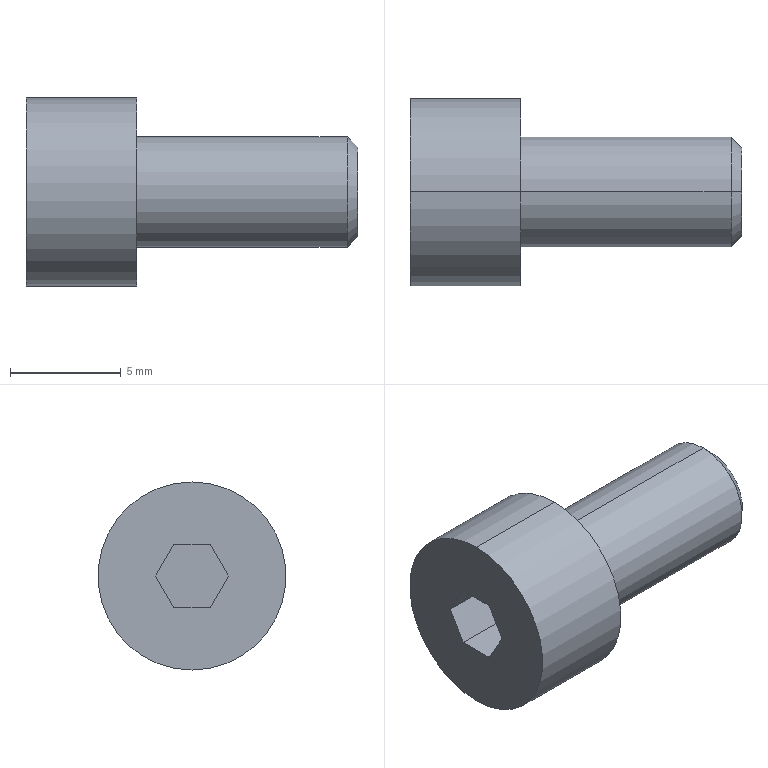Part | STEP file | _DBA01-D50-d20-e22-005 | 1 solid | 16 faces | box 15 x 8.5 x 8.5 mm | volume 460.635 mm3 | plane 10 | cylinder 4 | cone 2 | commonest cylinder face diameters 5 x2 8.5 x2
STEP:
#1=CARTESIAN_POINT('',(5.,0.,-2.5));
#2=VERTEX_POINT('',#1);
#3=CARTESIAN_POINT('',(5.,0.,2.5));
#4=VERTEX_POINT('',#3);
#5=CARTESIAN_POINT('',(5.,0.,0.));
#6=DIRECTION('',(-1.,0.,0.));
#7=DIRECTION('',(0.,0.,1.));
#8=AXIS2_PLACEMENT_3D('',#5,#6,#7);
#9=CIRCLE('',#8,2.5);
#10=EDGE_CURVE('',#2,#4,#9,.T.);
#11=ORIENTED_EDGE('',*,*,#10,.F.);
#12=CARTESIAN_POINT('',(14.509,0.,-2.5));
#13=VERTEX_POINT('',#12);
#14=CARTESIAN_POINT('',(0.,0.,-2.5));
#15=DIRECTION('',(1.,0.,0.));
#16=VECTOR('',#15,1000.);
#17=LINE('',#14,#16);
#18=EDGE_CURVE('',#2,#13,#17,.T.);
#19=ORIENTED_EDGE('',*,*,#18,.T.);
#20=CARTESIAN_POINT('',(14.509,0.,2.5));
#21=VERTEX_POINT('',#20);
#22=CARTESIAN_POINT('',(14.509,0.,0.));
#23=DIRECTION('',(-1.,0.,0.));
#24=DIRECTION('',(0.,0.,1.));
#25=AXIS2_PLACEMENT_3D('',#22,#23,#24);
#26=CIRCLE('',#25,2.5);
#27=EDGE_CURVE('',#13,#21,#26,.T.);
#28=ORIENTED_EDGE('',*,*,#27,.T.);
#29=CARTESIAN_POINT('',(0.,0.,2.5));
#30=DIRECTION('',(1.,0.,0.));
#31=VECTOR('',#30,1000.);
#32=LINE('',#29,#31);
#33=EDGE_CURVE('',#4,#21,#32,.T.);
#34=ORIENTED_EDGE('',*,*,#33,.F.);
#35=EDGE_LOOP('',(#11,#19,#28,#34));
#36=FACE_OUTER_BOUND('',#35,.T.);
#37=CARTESIAN_POINT('',(0.,0.,0.));
#38=DIRECTION('',(1.,0.,0.));
#39=DIRECTION('',(0.,0.,1.));
#40=AXIS2_PLACEMENT_3D('',#37,#38,#39);
#41=CYLINDRICAL_SURFACE('',#40,2.5);
#42=ADVANCED_FACE('',(#36),#41,.T.);
#43=CARTESIAN_POINT('',(0.,0.,-4.25));
#44=VERTEX_POINT('',#43);
#45=CARTESIAN_POINT('',(0.,0.,4.25));
#46=VERTEX_POINT('',#45);
#47=CARTESIAN_POINT('',(0.,0.,0.));
#48=DIRECTION('',(-1.,0.,0.));
#49=DIRECTION('',(0.,0.,1.));
#50=AXIS2_PLACEMENT_3D('',#47,#48,#49);
#51=CIRCLE('',#50,4.25);
#52=EDGE_CURVE('',#44,#46,#51,.T.);
#53=ORIENTED_EDGE('',*,*,#52,.F.);
#54=CARTESIAN_POINT('',(5.,0.,-4.25));
#55=VERTEX_POINT('',#54);
#56=CARTESIAN_POINT('',(0.,0.,-4.25));
#57=DIRECTION('',(1.,0.,0.));
#58=VECTOR('',#57,1000.);
#59=LINE('',#56,#58);
#60=EDGE_CURVE('',#44,#55,#59,.T.);
#61=ORIENTED_EDGE('',*,*,#60,.T.);
#62=CARTESIAN_POINT('',(5.,0.,4.25));
#63=VERTEX_POINT('',#62);
#64=CARTESIAN_POINT('',(5.,0.,0.));
#65=DIRECTION('',(-1.,0.,0.));
#66=DIRECTION('',(0.,0.,1.));
#67=AXIS2_PLACEMENT_3D('',#64,#65,#66);
#68=CIRCLE('',#67,4.25);
#69=EDGE_CURVE('',#55,#63,#68,.T.);
#70=ORIENTED_EDGE('',*,*,#69,.T.);
#71=CARTESIAN_POINT('',(0.,0.,4.25));
#72=DIRECTION('',(1.,0.,0.));
#73=VECTOR('',#72,1000.);
#74=LINE('',#71,#73);
#75=EDGE_CURVE('',#46,#63,#74,.T.);
#76=ORIENTED_EDGE('',*,*,#75,.F.);
#77=EDGE_LOOP('',(#53,#61,#70,#76));
#78=FACE_OUTER_BOUND('',#77,.T.);
#79=CARTESIAN_POINT('',(0.,0.,0.));
#80=DIRECTION('',(1.,0.,0.));
#81=DIRECTION('',(0.,0.,1.));
#82=AXIS2_PLACEMENT_3D('',#79,#80,#81);
#83=CYLINDRICAL_SURFACE('',#82,4.25);
#84=ADVANCED_FACE('',(#78),#83,.T.);
#85=CARTESIAN_POINT('',(15.,0.,2.01));
#86=VERTEX_POINT('',#85);
#87=CARTESIAN_POINT('',(15.,0.,-2.01));
#88=VERTEX_POINT('',#87);
#89=CARTESIAN_POINT('',(15.,0.,0.));
#90=DIRECTION('',(-1.,0.,0.));
#91=DIRECTION('',(0.,0.,1.));
#92=AXIS2_PLACEMENT_3D('',#89,#90,#91);
#93=CIRCLE('',#92,2.01);
#94=EDGE_CURVE('',#86,#88,#93,.T.);
#95=ORIENTED_EDGE('',*,*,#94,.T.);
#96=CARTESIAN_POINT('',(15.,0.,-2.01));
#97=DIRECTION('',(-0.7071,0.,-0.7071));
#98=VECTOR('',#97,1000.);
#99=LINE('',#96,#98);
#100=EDGE_CURVE('',#88,#13,#99,.T.);
#101=ORIENTED_EDGE('',*,*,#100,.T.);
#102=CARTESIAN_POINT('',(14.509,0.,0.));
#103=DIRECTION('',(-1.,0.,0.));
#104=DIRECTION('',(0.,0.,1.));
#105=AXIS2_PLACEMENT_3D('',#102,#103,#104);
#106=CIRCLE('',#105,2.5);
#107=EDGE_CURVE('',#21,#13,#106,.T.);
#108=ORIENTED_EDGE('',*,*,#107,.F.);
#109=CARTESIAN_POINT('',(15.,0.,2.01));
#110=DIRECTION('',(-0.7071,0.,0.7071));
#111=VECTOR('',#110,1000.);
#112=LINE('',#109,#111);
#113=EDGE_CURVE('',#86,#21,#112,.T.);
#114=ORIENTED_EDGE('',*,*,#113,.F.);
#115=EDGE_LOOP('',(#95,#101,#108,#114));
#116=FACE_OUTER_BOUND('',#115,.T.);
#117=CARTESIAN_POINT('',(15.,0.,0.));
#118=DIRECTION('',(-1.,0.,0.));
#119=DIRECTION('',(0.,0.,1.));
#120=AXIS2_PLACEMENT_3D('',#117,#118,#119);
#121=CONICAL_SURFACE('',#120,2.01,0.7854);
#122=ADVANCED_FACE('',(#116),#121,.T.);
#123=ORIENTED_EDGE('',*,*,#100,.F.);
#124=CARTESIAN_POINT('',(15.,0.,0.));
#125=DIRECTION('',(-1.,0.,0.));
#126=DIRECTION('',(0.,0.,1.));
#127=AXIS2_PLACEMENT_3D('',#124,#125,#126);
#128=CIRCLE('',#127,2.01);
#129=EDGE_CURVE('',#88,#86,#128,.T.);
#130=ORIENTED_EDGE('',*,*,#129,.T.);
#131=ORIENTED_EDGE('',*,*,#113,.T.);
#132=ORIENTED_EDGE('',*,*,#27,.F.);
#133=EDGE_LOOP('',(#123,#130,#131,#132));
#134=FACE_OUTER_BOUND('',#133,.T.);
#135=CARTESIAN_POINT('',(15.,0.,0.));
#136=DIRECTION('',(-1.,0.,0.));
#137=DIRECTION('',(0.,0.,1.));
#138=AXIS2_PLACEMENT_3D('',#135,#136,#137);
#139=CONICAL_SURFACE('',#138,2.01,0.7854);
#140=ADVANCED_FACE('',(#134),#139,.T.);
#141=ORIENTED_EDGE('',*,*,#94,.F.);
#142=ORIENTED_EDGE('',*,*,#129,.F.);
#143=EDGE_LOOP('',(#141,#142));
#144=FACE_OUTER_BOUND('',#143,.T.);
#145=CARTESIAN_POINT('',(15.,0.,0.));
#146=DIRECTION('',(-1.,0.,0.));
#147=DIRECTION('',(0.,0.,1.));
#148=AXIS2_PLACEMENT_3D('',#145,#146,#147);
#149=PLANE('',#148);
#150=ADVANCED_FACE('',(#144),#149,.F.);
#151=CARTESIAN_POINT('',(0.,0.,0.));
#152=DIRECTION('',(-1.,0.,0.));
#153=DIRECTION('',(0.,0.,1.));
#154=AXIS2_PLACEMENT_3D('',#151,#152,#153);
#155=CIRCLE('',#154,4.25);
#156=EDGE_CURVE('',#46,#44,#155,.T.);
#157=ORIENTED_EDGE('',*,*,#156,.T.);
#158=ORIENTED_EDGE('',*,*,#52,.T.);
#159=EDGE_LOOP('',(#157,#158));
#160=FACE_OUTER_BOUND('',#159,.T.);
#161=CARTESIAN_POINT('',(0.,-0.8248,1.429));
#162=VERTEX_POINT('',#161);
#163=CARTESIAN_POINT('',(0.,-1.65,0.));
#164=VERTEX_POINT('',#163);
#165=CARTESIAN_POINT('',(0.,-0.8248,1.429));
#166=DIRECTION('',(0.,-0.5,-0.866));
#167=VECTOR('',#166,1000.);
#168=LINE('',#165,#167);
#169=EDGE_CURVE('',#162,#164,#168,.T.);
#170=ORIENTED_EDGE('',*,*,#169,.T.);
#171=CARTESIAN_POINT('',(0.,-0.8248,-1.429));
#172=VERTEX_POINT('',#171);
#173=CARTESIAN_POINT('',(0.,-1.65,0.));
#174=DIRECTION('',(0.,0.5,-0.866));
#175=VECTOR('',#174,1000.);
#176=LINE('',#173,#175);
#177=EDGE_CURVE('',#164,#172,#176,.T.);
#178=ORIENTED_EDGE('',*,*,#177,.T.);
#179=CARTESIAN_POINT('',(0.,0.8248,-1.429));
#180=VERTEX_POINT('',#179);
#181=CARTESIAN_POINT('',(0.,-0.8248,-1.429));
#182=DIRECTION('',(0.,1.,0.));
#183=VECTOR('',#182,1000.);
#184=LINE('',#181,#183);
#185=EDGE_CURVE('',#172,#180,#184,.T.);
#186=ORIENTED_EDGE('',*,*,#185,.T.);
#187=CARTESIAN_POINT('',(0.,1.65,0.));
#188=VERTEX_POINT('',#187);
#189=CARTESIAN_POINT('',(0.,0.8248,-1.429));
#190=DIRECTION('',(0.,0.5,0.866));
#191=VECTOR('',#190,1000.);
#192=LINE('',#189,#191);
#193=EDGE_CURVE('',#180,#188,#192,.T.);
#194=ORIENTED_EDGE('',*,*,#193,.T.);
#195=CARTESIAN_POINT('',(0.,0.8248,1.429));
#196=VERTEX_POINT('',#195);
#197=CARTESIAN_POINT('',(0.,1.65,0.));
#198=DIRECTION('',(0.,-0.5,0.866));
#199=VECTOR('',#198,1000.);
#200=LINE('',#197,#199);
#201=EDGE_CURVE('',#188,#196,#200,.T.);
#202=ORIENTED_EDGE('',*,*,#201,.T.);
#203=CARTESIAN_POINT('',(0.,0.8248,1.429));
#204=DIRECTION('',(0.,-1.,0.));
#205=VECTOR('',#204,1000.);
#206=LINE('',#203,#205);
#207=EDGE_CURVE('',#196,#162,#206,.T.);
#208=ORIENTED_EDGE('',*,*,#207,.T.);
#209=EDGE_LOOP('',(#170,#178,#186,#194,#202,#208));
#210=FACE_BOUND('',#209,.T.);
#211=CARTESIAN_POINT('',(0.,-4.25,0.));
#212=DIRECTION('',(1.,0.,0.));
#213=DIRECTION('',(0.,1.,0.));
#214=AXIS2_PLACEMENT_3D('',#211,#212,#213);
#215=PLANE('',#214);
#216=ADVANCED_FACE('',(#160,#210),#215,.F.);
#217=ORIENTED_EDGE('',*,*,#60,.F.);
#218=ORIENTED_EDGE('',*,*,#156,.F.);
#219=ORIENTED_EDGE('',*,*,#75,.T.);
#220=CARTESIAN_POINT('',(5.,0.,0.));
#221=DIRECTION('',(-1.,0.,0.));
#222=DIRECTION('',(0.,0.,1.));
#223=AXIS2_PLACEMENT_3D('',#220,#221,#222);
#224=CIRCLE('',#223,4.25);
#225=EDGE_CURVE('',#63,#55,#224,.T.);
#226=ORIENTED_EDGE('',*,*,#225,.T.);
#227=EDGE_LOOP('',(#217,#218,#219,#226));
#228=FACE_OUTER_BOUND('',#227,.T.);
#229=CARTESIAN_POINT('',(0.,0.,0.));
#230=DIRECTION('',(1.,0.,0.));
#231=DIRECTION('',(0.,0.,1.));
#232=AXIS2_PLACEMENT_3D('',#229,#230,#231);
#233=CYLINDRICAL_SURFACE('',#232,4.25);
#234=ADVANCED_FACE('',(#228),#233,.T.);
#235=ORIENTED_EDGE('',*,*,#225,.F.);
#236=ORIENTED_EDGE('',*,*,#69,.F.);
#237=EDGE_LOOP('',(#235,#236));
#238=FACE_OUTER_BOUND('',#237,.T.);
#239=CARTESIAN_POINT('',(5.,0.,0.));
#240=DIRECTION('',(-1.,0.,0.));
#241=DIRECTION('',(0.,0.,1.));
#242=AXIS2_PLACEMENT_3D('',#239,#240,#241);
#243=CIRCLE('',#242,2.5);
#244=EDGE_CURVE('',#4,#2,#243,.T.);
#245=ORIENTED_EDGE('',*,*,#244,.T.);
#246=ORIENTED_EDGE('',*,*,#10,.T.);
#247=EDGE_LOOP('',(#245,#246));
#248=FACE_BOUND('',#247,.T.);
#249=CARTESIAN_POINT('',(5.,-2.5,0.));
#250=DIRECTION('',(-1.,0.,0.));
#251=DIRECTION('',(0.,0.,1.));
#252=AXIS2_PLACEMENT_3D('',#249,#250,#251);
#253=PLANE('',#252);
#254=ADVANCED_FACE('',(#238,#248),#253,.F.);
#255=ORIENTED_EDGE('',*,*,#18,.F.);
#256=ORIENTED_EDGE('',*,*,#244,.F.);
#257=ORIENTED_EDGE('',*,*,#33,.T.);
#258=ORIENTED_EDGE('',*,*,#107,.T.);
#259=EDGE_LOOP('',(#255,#256,#257,#258));
#260=FACE_OUTER_BOUND('',#259,.T.);
#261=CARTESIAN_POINT('',(0.,0.,0.));
#262=DIRECTION('',(1.,0.,0.));
#263=DIRECTION('',(0.,0.,1.));
#264=AXIS2_PLACEMENT_3D('',#261,#262,#263);
#265=CYLINDRICAL_SURFACE('',#264,2.5);
#266=ADVANCED_FACE('',(#260),#265,.T.);
#267=ORIENTED_EDGE('',*,*,#207,.F.);
#268=CARTESIAN_POINT('',(2.5,0.8248,1.429));
#269=VERTEX_POINT('',#268);
#270=CARTESIAN_POINT('',(2.5,0.8248,1.429));
#271=DIRECTION('',(-1.,0.,0.));
#272=VECTOR('',#271,1000.);
#273=LINE('',#270,#272);
#274=EDGE_CURVE('',#269,#196,#273,.T.);
#275=ORIENTED_EDGE('',*,*,#274,.F.);
#276=CARTESIAN_POINT('',(2.5,-0.8248,1.429));
#277=VERTEX_POINT('',#276);
#278=CARTESIAN_POINT('',(2.5,0.8248,1.429));
#279=DIRECTION('',(0.,-1.,0.));
#280=VECTOR('',#279,1000.);
#281=LINE('',#278,#280);
#282=EDGE_CURVE('',#269,#277,#281,.T.);
#283=ORIENTED_EDGE('',*,*,#282,.T.);
#284=CARTESIAN_POINT('',(2.5,-0.8248,1.429));
#285=DIRECTION('',(-1.,0.,0.));
#286=VECTOR('',#285,1000.);
#287=LINE('',#284,#286);
#288=EDGE_CURVE('',#277,#162,#287,.T.);
#289=ORIENTED_EDGE('',*,*,#288,.T.);
#290=EDGE_LOOP('',(#267,#275,#283,#289));
#291=FACE_OUTER_BOUND('',#290,.T.);
#292=CARTESIAN_POINT('',(2.5,0.8248,1.429));
#293=DIRECTION('',(0.,0.,-1.));
#294=DIRECTION('',(0.,-1.,0.));
#295=AXIS2_PLACEMENT_3D('',#292,#293,#294);
#296=PLANE('',#295);
#297=ADVANCED_FACE('',(#291),#296,.T.);
#298=ORIENTED_EDGE('',*,*,#169,.F.);
#299=ORIENTED_EDGE('',*,*,#288,.F.);
#300=CARTESIAN_POINT('',(2.5,-1.65,0.));
#301=VERTEX_POINT('',#300);
#302=CARTESIAN_POINT('',(2.5,-0.8248,1.429));
#303=DIRECTION('',(0.,-0.5,-0.866));
#304=VECTOR('',#303,1000.);
#305=LINE('',#302,#304);
#306=EDGE_CURVE('',#277,#301,#305,.T.);
#307=ORIENTED_EDGE('',*,*,#306,.T.);
#308=CARTESIAN_POINT('',(2.5,-1.65,0.));
#309=DIRECTION('',(-1.,0.,0.));
#310=VECTOR('',#309,1000.);
#311=LINE('',#308,#310);
#312=EDGE_CURVE('',#301,#164,#311,.T.);
#313=ORIENTED_EDGE('',*,*,#312,.T.);
#314=EDGE_LOOP('',(#298,#299,#307,#313));
#315=FACE_OUTER_BOUND('',#314,.T.);
#316=CARTESIAN_POINT('',(2.5,-0.8248,1.429));
#317=DIRECTION('',(0.,0.866,-0.5));
#318=DIRECTION('',(-1.,0.,0.));
#319=AXIS2_PLACEMENT_3D('',#316,#317,#318);
#320=PLANE('',#319);
#321=ADVANCED_FACE('',(#315),#320,.T.);
#322=ORIENTED_EDGE('',*,*,#177,.F.);
#323=ORIENTED_EDGE('',*,*,#312,.F.);
#324=CARTESIAN_POINT('',(2.5,-0.8248,-1.429));
#325=VERTEX_POINT('',#324);
#326=CARTESIAN_POINT('',(2.5,-1.65,0.));
#327=DIRECTION('',(0.,0.5,-0.866));
#328=VECTOR('',#327,1000.);
#329=LINE('',#326,#328);
#330=EDGE_CURVE('',#301,#325,#329,.T.);
#331=ORIENTED_EDGE('',*,*,#330,.T.);
#332=CARTESIAN_POINT('',(2.5,-0.8248,-1.429));
#333=DIRECTION('',(-1.,0.,0.));
#334=VECTOR('',#333,1000.);
#335=LINE('',#332,#334);
#336=EDGE_CURVE('',#325,#172,#335,.T.);
#337=ORIENTED_EDGE('',*,*,#336,.T.);
#338=EDGE_LOOP('',(#322,#323,#331,#337));
#339=FACE_OUTER_BOUND('',#338,.T.);
#340=CARTESIAN_POINT('',(2.5,-1.65,0.));
#341=DIRECTION('',(0.,0.866,0.5));
#342=DIRECTION('',(1.,0.,0.));
#343=AXIS2_PLACEMENT_3D('',#340,#341,#342);
#344=PLANE('',#343);
#345=ADVANCED_FACE('',(#339),#344,.T.);
#346=ORIENTED_EDGE('',*,*,#185,.F.);
#347=ORIENTED_EDGE('',*,*,#336,.F.);
#348=CARTESIAN_POINT('',(2.5,0.8248,-1.429));
#349=VERTEX_POINT('',#348);
#350=CARTESIAN_POINT('',(2.5,-0.8248,-1.429));
#351=DIRECTION('',(0.,1.,0.));
#352=VECTOR('',#351,1000.);
#353=LINE('',#350,#352);
#354=EDGE_CURVE('',#325,#349,#353,.T.);
#355=ORIENTED_EDGE('',*,*,#354,.T.);
#356=CARTESIAN_POINT('',(2.5,0.8248,-1.429));
#357=DIRECTION('',(-1.,0.,0.));
#358=VECTOR('',#357,1000.);
#359=LINE('',#356,#358);
#360=EDGE_CURVE('',#349,#180,#359,.T.);
#361=ORIENTED_EDGE('',*,*,#360,.T.);
#362=EDGE_LOOP('',(#346,#347,#355,#361));
#363=FACE_OUTER_BOUND('',#362,.T.);
#364=CARTESIAN_POINT('',(2.5,-0.8248,-1.429));
#365=DIRECTION('',(0.,0.,1.));
#366=DIRECTION('',(1.,0.,0.));
#367=AXIS2_PLACEMENT_3D('',#364,#365,#366);
#368=PLANE('',#367);
#369=ADVANCED_FACE('',(#363),#368,.T.);
#370=ORIENTED_EDGE('',*,*,#193,.F.);
#371=ORIENTED_EDGE('',*,*,#360,.F.);
#372=CARTESIAN_POINT('',(2.5,1.65,0.));
#373=VERTEX_POINT('',#372);
#374=CARTESIAN_POINT('',(2.5,0.8248,-1.429));
#375=DIRECTION('',(0.,0.5,0.866));
#376=VECTOR('',#375,1000.);
#377=LINE('',#374,#376);
#378=EDGE_CURVE('',#349,#373,#377,.T.);
#379=ORIENTED_EDGE('',*,*,#378,.T.);
#380=CARTESIAN_POINT('',(2.5,1.65,0.));
#381=DIRECTION('',(-1.,0.,0.));
#382=VECTOR('',#381,1000.);
#383=LINE('',#380,#382);
#384=EDGE_CURVE('',#373,#188,#383,.T.);
#385=ORIENTED_EDGE('',*,*,#384,.T.);
#386=EDGE_LOOP('',(#370,#371,#379,#385));
#387=FACE_OUTER_BOUND('',#386,.T.);
#388=CARTESIAN_POINT('',(2.5,0.8248,-1.429));
#389=DIRECTION('',(0.,-0.866,0.5));
#390=DIRECTION('',(-1.,0.,0.));
#391=AXIS2_PLACEMENT_3D('',#388,#389,#390);
#392=PLANE('',#391);
#393=ADVANCED_FACE('',(#387),#392,.T.);
#394=ORIENTED_EDGE('',*,*,#201,.F.);
#395=ORIENTED_EDGE('',*,*,#384,.F.);
#396=CARTESIAN_POINT('',(2.5,1.65,0.));
#397=DIRECTION('',(0.,-0.5,0.866));
#398=VECTOR('',#397,1000.);
#399=LINE('',#396,#398);
#400=EDGE_CURVE('',#373,#269,#399,.T.);
#401=ORIENTED_EDGE('',*,*,#400,.T.);
#402=ORIENTED_EDGE('',*,*,#274,.T.);
#403=EDGE_LOOP('',(#394,#395,#401,#402));
#404=FACE_OUTER_BOUND('',#403,.T.);
#405=CARTESIAN_POINT('',(2.5,1.65,0.));
#406=DIRECTION('',(0.,-0.866,-0.5));
#407=DIRECTION('',(0.,0.5,-0.866));
#408=AXIS2_PLACEMENT_3D('',#405,#406,#407);
#409=PLANE('',#408);
#410=ADVANCED_FACE('',(#404),#409,.T.);
#411=ORIENTED_EDGE('',*,*,#282,.F.);
#412=ORIENTED_EDGE('',*,*,#400,.F.);
#413=ORIENTED_EDGE('',*,*,#378,.F.);
#414=ORIENTED_EDGE('',*,*,#354,.F.);
#415=ORIENTED_EDGE('',*,*,#330,.F.);
#416=ORIENTED_EDGE('',*,*,#306,.F.);
#417=EDGE_LOOP('',(#411,#412,#413,#414,#415,#416));
#418=FACE_OUTER_BOUND('',#417,.T.);
#419=CARTESIAN_POINT('',(2.5,0.,0.));
#420=DIRECTION('',(1.,0.,0.));
#421=DIRECTION('',(0.,1.,0.));
#422=AXIS2_PLACEMENT_3D('',#419,#420,#421);
#423=PLANE('',#422);
#424=ADVANCED_FACE('',(#418),#423,.F.);
#425=CLOSED_SHELL('',(#42,#84,#122,#140,#150,#216,#234,#254,#266,#297,#321,#345,#369,#393,#410,#424));
#426=MANIFOLD_SOLID_BREP('',#425);
#427=CARTESIAN_POINT('',(0.,0.,0.));
#428=DIRECTION('',(0.,0.,1.));
#429=DIRECTION('',(1.,0.,0.));
#430=AXIS2_PLACEMENT_3D('',#427,#428,#429);
#431=(LENGTH_UNIT()NAMED_UNIT(*)SI_UNIT(.MILLI.,.METRE.));
#432=UNCERTAINTY_MEASURE_WITH_UNIT(LENGTH_MEASURE(0.00001),#431,'','');
#433=(NAMED_UNIT(*)PLANE_ANGLE_UNIT()SI_UNIT($,.RADIAN.));
#434=(NAMED_UNIT(*)SI_UNIT($,.STERADIAN.)SOLID_ANGLE_UNIT());
#435=(GEOMETRIC_REPRESENTATION_CONTEXT(3)GLOBAL_UNCERTAINTY_ASSIGNED_CONTEXT((#432))GLOBAL_UNIT_ASSIGNED_CONTEXT((#431,#433,#434))REPRESENTATION_CONTEXT('',''));
#436=ADVANCED_BREP_SHAPE_REPRESENTATION('',(#426,#430),#435);